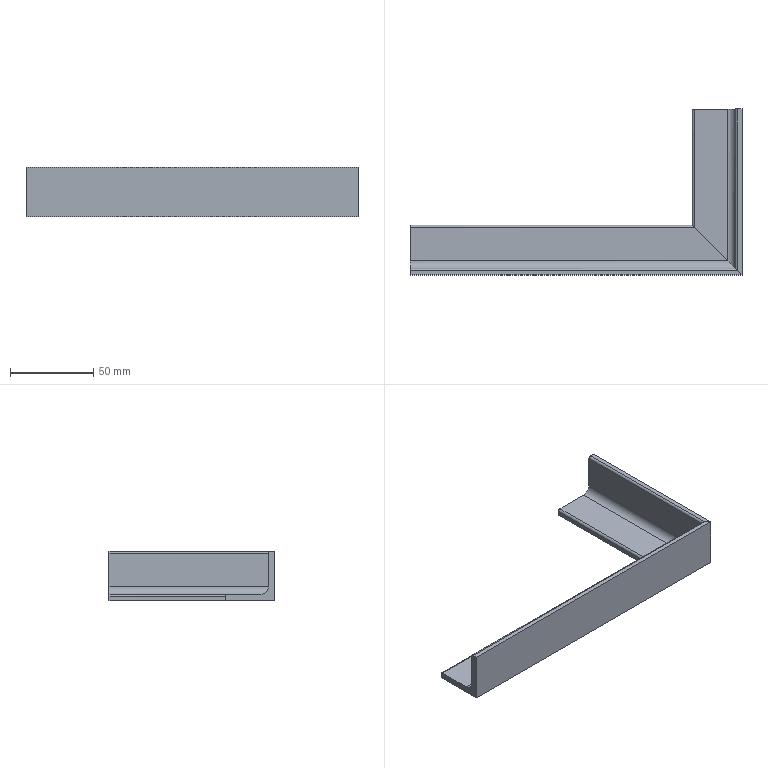Part | SolidWorks | features WeldMemberFeat 1, WeldmentFeature 1 | 2 solids | 22 faces | box 200 x 100 x 30 mm | volume 64241 mm3 | plane 16 | cylinder 6 | commonest cylinder face diameters 2.667 x4 9 x2
STEP:
#1=CARTESIAN_POINT('',(200.,0.,0.));
#2=VERTEX_POINT('',#1);
#3=CARTESIAN_POINT('',(170.,30.,0.));
#4=VERTEX_POINT('',#3);
#5=CARTESIAN_POINT('',(185.,15.,0.));
#6=DIRECTION('',(-0.7071,0.7071,0.));
#7=VECTOR('',#6,1000.);
#8=LINE('',#5,#7);
#9=EDGE_CURVE('',#2,#4,#8,.T.);
#10=ORIENTED_EDGE('',*,*,#9,.F.);
#11=CARTESIAN_POINT('',(0.,0.,0.));
#12=VERTEX_POINT('',#11);
#13=CARTESIAN_POINT('',(200.,0.,0.));
#14=DIRECTION('',(-1.,0.,0.));
#15=VECTOR('',#14,1000.);
#16=LINE('',#13,#15);
#17=EDGE_CURVE('',#2,#12,#16,.T.);
#18=ORIENTED_EDGE('',*,*,#17,.T.);
#19=CARTESIAN_POINT('',(0.,30.,0.));
#20=VERTEX_POINT('',#19);
#21=CARTESIAN_POINT('',(0.,30.,0.));
#22=DIRECTION('',(0.,1.,0.));
#23=VECTOR('',#22,1000.);
#24=LINE('',#21,#23);
#25=EDGE_CURVE('',#12,#20,#24,.T.);
#26=ORIENTED_EDGE('',*,*,#25,.T.);
#27=CARTESIAN_POINT('',(200.,30.,0.));
#28=DIRECTION('',(-1.,0.,0.));
#29=VECTOR('',#28,1000.);
#30=LINE('',#27,#29);
#31=EDGE_CURVE('',#4,#20,#30,.T.);
#32=ORIENTED_EDGE('',*,*,#31,.F.);
#33=EDGE_LOOP('',(#10,#18,#26,#32));
#34=FACE_OUTER_BOUND('',#33,.T.);
#35=CARTESIAN_POINT('',(200.,30.,0.));
#36=DIRECTION('',(0.,0.,1.));
#37=DIRECTION('',(1.,0.,0.));
#38=AXIS2_PLACEMENT_3D('',#35,#36,#37);
#39=PLANE('',#38);
#40=ADVANCED_FACE('',(#34),#39,.F.);
#41=CARTESIAN_POINT('',(170.,30.,2.667));
#42=VERTEX_POINT('',#41);
#43=CARTESIAN_POINT('',(170.,30.,0.));
#44=DIRECTION('',(0.,0.,1.));
#45=VECTOR('',#44,1000.);
#46=LINE('',#43,#45);
#47=EDGE_CURVE('',#4,#42,#46,.T.);
#48=ORIENTED_EDGE('',*,*,#47,.F.);
#49=ORIENTED_EDGE('',*,*,#31,.T.);
#50=CARTESIAN_POINT('',(0.,30.,2.667));
#51=VERTEX_POINT('',#50);
#52=CARTESIAN_POINT('',(0.,30.,0.));
#53=DIRECTION('',(0.,0.,1.));
#54=VECTOR('',#53,1000.);
#55=LINE('',#52,#54);
#56=EDGE_CURVE('',#20,#51,#55,.T.);
#57=ORIENTED_EDGE('',*,*,#56,.T.);
#58=CARTESIAN_POINT('',(200.,30.,2.667));
#59=DIRECTION('',(-1.,0.,0.));
#60=VECTOR('',#59,1000.);
#61=LINE('',#58,#60);
#62=EDGE_CURVE('',#42,#51,#61,.T.);
#63=ORIENTED_EDGE('',*,*,#62,.F.);
#64=EDGE_LOOP('',(#48,#49,#57,#63));
#65=FACE_OUTER_BOUND('',#64,.T.);
#66=CARTESIAN_POINT('',(200.,30.,0.));
#67=DIRECTION('',(0.,-1.,0.));
#68=DIRECTION('',(0.,0.,-1.));
#69=AXIS2_PLACEMENT_3D('',#66,#67,#68);
#70=PLANE('',#69);
#71=ADVANCED_FACE('',(#65),#70,.F.);
#72=CARTESIAN_POINT('',(171.333,28.667,4.));
#73=VERTEX_POINT('',#72);
#74=CARTESIAN_POINT('',(170.,30.,2.667));
#75=CARTESIAN_POINT('',(170.,30.,3.448));
#76=CARTESIAN_POINT('',(170.552,29.448,4.));
#77=CARTESIAN_POINT('',(171.333,28.667,4.));
#78=(BOUNDED_CURVE()B_SPLINE_CURVE(3,(#74,#75,#76,#77),.UNSPECIFIED.,.F.,.T.)B_SPLINE_CURVE_WITH_KNOTS((4,4),(0.,1.571),.UNSPECIFIED.)CURVE()GEOMETRIC_REPRESENTATION_ITEM()RATIONAL_B_SPLINE_CURVE((1.,0.8047,0.8047,1.))REPRESENTATION_ITEM(''));
#79=EDGE_CURVE('',#42,#73,#78,.T.);
#80=ORIENTED_EDGE('',*,*,#79,.F.);
#81=ORIENTED_EDGE('',*,*,#62,.T.);
#82=CARTESIAN_POINT('',(0.,28.667,4.));
#83=VERTEX_POINT('',#82);
#84=CARTESIAN_POINT('',(0.,28.667,2.667));
#85=DIRECTION('',(1.,0.,0.));
#86=DIRECTION('',(0.,0.,-1.));
#87=AXIS2_PLACEMENT_3D('',#84,#85,#86);
#88=CIRCLE('',#87,1.333);
#89=EDGE_CURVE('',#51,#83,#88,.T.);
#90=ORIENTED_EDGE('',*,*,#89,.T.);
#91=CARTESIAN_POINT('',(200.,28.667,4.));
#92=DIRECTION('',(-1.,0.,0.));
#93=VECTOR('',#92,1000.);
#94=LINE('',#91,#93);
#95=EDGE_CURVE('',#73,#83,#94,.T.);
#96=ORIENTED_EDGE('',*,*,#95,.F.);
#97=EDGE_LOOP('',(#80,#81,#90,#96));
#98=FACE_OUTER_BOUND('',#97,.T.);
#99=CARTESIAN_POINT('',(200.,28.667,2.667));
#100=DIRECTION('',(-1.,0.,0.));
#101=DIRECTION('',(0.,0.,1.));
#102=AXIS2_PLACEMENT_3D('',#99,#100,#101);
#103=CYLINDRICAL_SURFACE('',#102,1.333);
#104=ADVANCED_FACE('',(#98),#103,.T.);
#105=CARTESIAN_POINT('',(191.5,8.5,4.));
#106=VERTEX_POINT('',#105);
#107=CARTESIAN_POINT('',(195.75,4.25,4.));
#108=DIRECTION('',(0.7071,-0.7071,0.));
#109=VECTOR('',#108,1000.);
#110=LINE('',#107,#109);
#111=EDGE_CURVE('',#73,#106,#110,.T.);
#112=ORIENTED_EDGE('',*,*,#111,.F.);
#113=ORIENTED_EDGE('',*,*,#95,.T.);
#114=CARTESIAN_POINT('',(0.,8.5,4.));
#115=VERTEX_POINT('',#114);
#116=CARTESIAN_POINT('',(0.,8.5,4.));
#117=DIRECTION('',(0.,-1.,0.));
#118=VECTOR('',#117,1000.);
#119=LINE('',#116,#118);
#120=EDGE_CURVE('',#83,#115,#119,.T.);
#121=ORIENTED_EDGE('',*,*,#120,.T.);
#122=CARTESIAN_POINT('',(200.,8.5,4.));
#123=DIRECTION('',(-1.,0.,0.));
#124=VECTOR('',#123,1000.);
#125=LINE('',#122,#124);
#126=EDGE_CURVE('',#106,#115,#125,.T.);
#127=ORIENTED_EDGE('',*,*,#126,.F.);
#128=EDGE_LOOP('',(#112,#113,#121,#127));
#129=FACE_OUTER_BOUND('',#128,.T.);
#130=CARTESIAN_POINT('',(200.,8.5,4.));
#131=DIRECTION('',(0.,0.,-1.));
#132=DIRECTION('',(0.,1.,0.));
#133=AXIS2_PLACEMENT_3D('',#130,#131,#132);
#134=PLANE('',#133);
#135=ADVANCED_FACE('',(#129),#134,.F.);
#136=CARTESIAN_POINT('',(196.,4.,8.5));
#137=VERTEX_POINT('',#136);
#138=CARTESIAN_POINT('',(191.5,8.5,4.));
#139=CARTESIAN_POINT('',(194.136,5.864,4.));
#140=CARTESIAN_POINT('',(196.,4.,5.864));
#141=CARTESIAN_POINT('',(196.,4.,8.5));
#142=(BOUNDED_CURVE()B_SPLINE_CURVE(3,(#138,#139,#140,#141),.UNSPECIFIED.,.F.,.T.)B_SPLINE_CURVE_WITH_KNOTS((4,4),(1.571,3.142),.UNSPECIFIED.)CURVE()GEOMETRIC_REPRESENTATION_ITEM()RATIONAL_B_SPLINE_CURVE((1.,0.8047,0.8047,1.))REPRESENTATION_ITEM(''));
#143=EDGE_CURVE('',#106,#137,#142,.T.);
#144=ORIENTED_EDGE('',*,*,#143,.F.);
#145=ORIENTED_EDGE('',*,*,#126,.T.);
#146=CARTESIAN_POINT('',(0.,4.,8.5));
#147=VERTEX_POINT('',#146);
#148=CARTESIAN_POINT('',(0.,8.5,8.5));
#149=DIRECTION('',(-1.,0.,0.));
#150=DIRECTION('',(0.,0.,1.));
#151=AXIS2_PLACEMENT_3D('',#148,#149,#150);
#152=CIRCLE('',#151,4.5);
#153=EDGE_CURVE('',#115,#147,#152,.T.);
#154=ORIENTED_EDGE('',*,*,#153,.T.);
#155=CARTESIAN_POINT('',(200.,4.,8.5));
#156=DIRECTION('',(-1.,0.,0.));
#157=VECTOR('',#156,1000.);
#158=LINE('',#155,#157);
#159=EDGE_CURVE('',#137,#147,#158,.T.);
#160=ORIENTED_EDGE('',*,*,#159,.F.);
#161=EDGE_LOOP('',(#144,#145,#154,#160));
#162=FACE_OUTER_BOUND('',#161,.T.);
#163=CARTESIAN_POINT('',(200.,8.5,8.5));
#164=DIRECTION('',(-1.,0.,0.));
#165=DIRECTION('',(0.,0.,1.));
#166=AXIS2_PLACEMENT_3D('',#163,#164,#165);
#167=CYLINDRICAL_SURFACE('',#166,4.5);
#168=ADVANCED_FACE('',(#162),#167,.F.);
#169=CARTESIAN_POINT('',(196.,4.,28.667));
#170=VERTEX_POINT('',#169);
#171=CARTESIAN_POINT('',(196.,4.,28.667));
#172=DIRECTION('',(0.,0.,1.));
#173=VECTOR('',#172,1000.);
#174=LINE('',#171,#173);
#175=EDGE_CURVE('',#137,#170,#174,.T.);
#176=ORIENTED_EDGE('',*,*,#175,.F.);
#177=ORIENTED_EDGE('',*,*,#159,.T.);
#178=CARTESIAN_POINT('',(0.,4.,28.667));
#179=VERTEX_POINT('',#178);
#180=CARTESIAN_POINT('',(0.,4.,28.667));
#181=DIRECTION('',(0.,0.,1.));
#182=VECTOR('',#181,1000.);
#183=LINE('',#180,#182);
#184=EDGE_CURVE('',#147,#179,#183,.T.);
#185=ORIENTED_EDGE('',*,*,#184,.T.);
#186=CARTESIAN_POINT('',(200.,4.,28.667));
#187=DIRECTION('',(-1.,0.,0.));
#188=VECTOR('',#187,1000.);
#189=LINE('',#186,#188);
#190=EDGE_CURVE('',#170,#179,#189,.T.);
#191=ORIENTED_EDGE('',*,*,#190,.F.);
#192=EDGE_LOOP('',(#176,#177,#185,#191));
#193=FACE_OUTER_BOUND('',#192,.T.);
#194=CARTESIAN_POINT('',(200.,4.,28.667));
#195=DIRECTION('',(0.,-1.,0.));
#196=DIRECTION('',(0.,0.,-1.));
#197=AXIS2_PLACEMENT_3D('',#194,#195,#196);
#198=PLANE('',#197);
#199=ADVANCED_FACE('',(#193),#198,.F.);
#200=CARTESIAN_POINT('',(197.333,2.667,30.));
#201=VERTEX_POINT('',#200);
#202=CARTESIAN_POINT('',(196.,4.,28.667));
#203=CARTESIAN_POINT('',(196.,4.,29.448));
#204=CARTESIAN_POINT('',(196.552,3.448,30.));
#205=CARTESIAN_POINT('',(197.333,2.667,30.));
#206=(BOUNDED_CURVE()B_SPLINE_CURVE(3,(#202,#203,#204,#205),.UNSPECIFIED.,.F.,.T.)B_SPLINE_CURVE_WITH_KNOTS((4,4),(0.,1.571),.UNSPECIFIED.)CURVE()GEOMETRIC_REPRESENTATION_ITEM()RATIONAL_B_SPLINE_CURVE((1.,0.8047,0.8047,1.))REPRESENTATION_ITEM(''));
#207=EDGE_CURVE('',#170,#201,#206,.T.);
#208=ORIENTED_EDGE('',*,*,#207,.F.);
#209=ORIENTED_EDGE('',*,*,#190,.T.);
#210=CARTESIAN_POINT('',(0.,2.667,30.));
#211=VERTEX_POINT('',#210);
#212=CARTESIAN_POINT('',(0.,2.667,28.667));
#213=DIRECTION('',(1.,0.,0.));
#214=DIRECTION('',(0.,0.,1.));
#215=AXIS2_PLACEMENT_3D('',#212,#213,#214);
#216=CIRCLE('',#215,1.333);
#217=EDGE_CURVE('',#179,#211,#216,.T.);
#218=ORIENTED_EDGE('',*,*,#217,.T.);
#219=CARTESIAN_POINT('',(200.,2.667,30.));
#220=DIRECTION('',(-1.,0.,0.));
#221=VECTOR('',#220,1000.);
#222=LINE('',#219,#221);
#223=EDGE_CURVE('',#201,#211,#222,.T.);
#224=ORIENTED_EDGE('',*,*,#223,.F.);
#225=EDGE_LOOP('',(#208,#209,#218,#224));
#226=FACE_OUTER_BOUND('',#225,.T.);
#227=CARTESIAN_POINT('',(200.,2.667,28.667));
#228=DIRECTION('',(-1.,0.,0.));
#229=DIRECTION('',(0.,0.,1.));
#230=AXIS2_PLACEMENT_3D('',#227,#228,#229);
#231=CYLINDRICAL_SURFACE('',#230,1.333);
#232=ADVANCED_FACE('',(#226),#231,.T.);
#233=CARTESIAN_POINT('',(200.,0.,30.));
#234=VERTEX_POINT('',#233);
#235=CARTESIAN_POINT('',(200.,0.,30.));
#236=DIRECTION('',(0.7071,-0.7071,0.));
#237=VECTOR('',#236,1000.);
#238=LINE('',#235,#237);
#239=EDGE_CURVE('',#201,#234,#238,.T.);
#240=ORIENTED_EDGE('',*,*,#239,.F.);
#241=ORIENTED_EDGE('',*,*,#223,.T.);
#242=CARTESIAN_POINT('',(0.,0.,30.));
#243=VERTEX_POINT('',#242);
#244=CARTESIAN_POINT('',(0.,0.,30.));
#245=DIRECTION('',(0.,-1.,0.));
#246=VECTOR('',#245,1000.);
#247=LINE('',#244,#246);
#248=EDGE_CURVE('',#211,#243,#247,.T.);
#249=ORIENTED_EDGE('',*,*,#248,.T.);
#250=CARTESIAN_POINT('',(200.,0.,30.));
#251=DIRECTION('',(-1.,0.,0.));
#252=VECTOR('',#251,1000.);
#253=LINE('',#250,#252);
#254=EDGE_CURVE('',#234,#243,#253,.T.);
#255=ORIENTED_EDGE('',*,*,#254,.F.);
#256=EDGE_LOOP('',(#240,#241,#249,#255));
#257=FACE_OUTER_BOUND('',#256,.T.);
#258=CARTESIAN_POINT('',(200.,0.,30.));
#259=DIRECTION('',(0.,0.,-1.));
#260=DIRECTION('',(-1.,0.,0.));
#261=AXIS2_PLACEMENT_3D('',#258,#259,#260);
#262=PLANE('',#261);
#263=ADVANCED_FACE('',(#257),#262,.F.);
#264=CARTESIAN_POINT('',(200.,0.,0.));
#265=DIRECTION('',(0.,0.,-1.));
#266=VECTOR('',#265,1000.);
#267=LINE('',#264,#266);
#268=EDGE_CURVE('',#234,#2,#267,.T.);
#269=ORIENTED_EDGE('',*,*,#268,.F.);
#270=ORIENTED_EDGE('',*,*,#254,.T.);
#271=CARTESIAN_POINT('',(0.,0.,0.));
#272=DIRECTION('',(0.,0.,-1.));
#273=VECTOR('',#272,1000.);
#274=LINE('',#271,#273);
#275=EDGE_CURVE('',#243,#12,#274,.T.);
#276=ORIENTED_EDGE('',*,*,#275,.T.);
#277=ORIENTED_EDGE('',*,*,#17,.F.);
#278=EDGE_LOOP('',(#269,#270,#276,#277));
#279=FACE_OUTER_BOUND('',#278,.T.);
#280=CARTESIAN_POINT('',(200.,0.,0.));
#281=DIRECTION('',(0.,1.,0.));
#282=DIRECTION('',(0.,0.,1.));
#283=AXIS2_PLACEMENT_3D('',#280,#281,#282);
#284=PLANE('',#283);
#285=ADVANCED_FACE('',(#279),#284,.F.);
#286=ORIENTED_EDGE('',*,*,#25,.F.);
#287=ORIENTED_EDGE('',*,*,#275,.F.);
#288=ORIENTED_EDGE('',*,*,#248,.F.);
#289=ORIENTED_EDGE('',*,*,#217,.F.);
#290=ORIENTED_EDGE('',*,*,#184,.F.);
#291=ORIENTED_EDGE('',*,*,#153,.F.);
#292=ORIENTED_EDGE('',*,*,#120,.F.);
#293=ORIENTED_EDGE('',*,*,#89,.F.);
#294=ORIENTED_EDGE('',*,*,#56,.F.);
#295=EDGE_LOOP('',(#286,#287,#288,#289,#290,#291,#292,#293,#294));
#296=FACE_OUTER_BOUND('',#295,.T.);
#297=CARTESIAN_POINT('',(0.,2.667,28.667));
#298=DIRECTION('',(-1.,0.,0.));
#299=DIRECTION('',(0.,0.,1.));
#300=AXIS2_PLACEMENT_3D('',#297,#298,#299);
#301=PLANE('',#300);
#302=ADVANCED_FACE('',(#296),#301,.T.);
#303=ORIENTED_EDGE('',*,*,#268,.T.);
#304=ORIENTED_EDGE('',*,*,#9,.T.);
#305=ORIENTED_EDGE('',*,*,#47,.T.);
#306=ORIENTED_EDGE('',*,*,#79,.T.);
#307=ORIENTED_EDGE('',*,*,#111,.T.);
#308=ORIENTED_EDGE('',*,*,#143,.T.);
#309=ORIENTED_EDGE('',*,*,#175,.T.);
#310=ORIENTED_EDGE('',*,*,#207,.T.);
#311=ORIENTED_EDGE('',*,*,#239,.T.);
#312=EDGE_LOOP('',(#303,#304,#305,#306,#307,#308,#309,#310,#311));
#313=FACE_OUTER_BOUND('',#312,.T.);
#314=CARTESIAN_POINT('',(200.,0.,0.));
#315=DIRECTION('',(0.7071,0.7071,0.));
#316=DIRECTION('',(-0.7071,0.7071,0.));
#317=AXIS2_PLACEMENT_3D('',#314,#315,#316);
#318=PLANE('',#317);
#319=ADVANCED_FACE('',(#313),#318,.T.);
#320=CLOSED_SHELL('',(#40,#71,#104,#135,#168,#199,#232,#263,#285,#302,#319));
#321=MANIFOLD_SOLID_BREP('',#320);
#322=CARTESIAN_POINT('',(170.,30.,0.));
#323=VERTEX_POINT('',#322);
#324=CARTESIAN_POINT('',(200.,0.,0.));
#325=VERTEX_POINT('',#324);
#326=CARTESIAN_POINT('',(135.,65.,0.));
#327=DIRECTION('',(0.7071,-0.7071,0.));
#328=VECTOR('',#327,1000.);
#329=LINE('',#326,#328);
#330=EDGE_CURVE('',#323,#325,#329,.T.);
#331=ORIENTED_EDGE('',*,*,#330,.F.);
#332=CARTESIAN_POINT('',(170.,100.,0.));
#333=VERTEX_POINT('',#332);
#334=CARTESIAN_POINT('',(170.,100.,0.));
#335=DIRECTION('',(0.,-1.,0.));
#336=VECTOR('',#335,1000.);
#337=LINE('',#334,#336);
#338=EDGE_CURVE('',#333,#323,#337,.T.);
#339=ORIENTED_EDGE('',*,*,#338,.F.);
#340=CARTESIAN_POINT('',(200.,100.,0.));
#341=VERTEX_POINT('',#340);
#342=CARTESIAN_POINT('',(170.,100.,0.));
#343=DIRECTION('',(-1.,0.,0.));
#344=VECTOR('',#343,1000.);
#345=LINE('',#342,#344);
#346=EDGE_CURVE('',#341,#333,#345,.T.);
#347=ORIENTED_EDGE('',*,*,#346,.F.);
#348=CARTESIAN_POINT('',(200.,100.,0.));
#349=DIRECTION('',(0.,-1.,0.));
#350=VECTOR('',#349,1000.);
#351=LINE('',#348,#350);
#352=EDGE_CURVE('',#341,#325,#351,.T.);
#353=ORIENTED_EDGE('',*,*,#352,.T.);
#354=EDGE_LOOP('',(#331,#339,#347,#353));
#355=FACE_OUTER_BOUND('',#354,.T.);
#356=CARTESIAN_POINT('',(170.,100.,0.));
#357=DIRECTION('',(0.,0.,1.));
#358=DIRECTION('',(1.,0.,0.));
#359=AXIS2_PLACEMENT_3D('',#356,#357,#358);
#360=PLANE('',#359);
#361=ADVANCED_FACE('',(#355),#360,.F.);
#362=CARTESIAN_POINT('',(170.,30.,2.667));
#363=VERTEX_POINT('',#362);
#364=CARTESIAN_POINT('',(170.,30.,0.));
#365=DIRECTION('',(0.,0.,-1.));
#366=VECTOR('',#365,1000.);
#367=LINE('',#364,#366);
#368=EDGE_CURVE('',#363,#323,#367,.T.);
#369=ORIENTED_EDGE('',*,*,#368,.F.);
#370=CARTESIAN_POINT('',(170.,100.,2.667));
#371=VERTEX_POINT('',#370);
#372=CARTESIAN_POINT('',(170.,100.,2.667));
#373=DIRECTION('',(0.,-1.,0.));
#374=VECTOR('',#373,1000.);
#375=LINE('',#372,#374);
#376=EDGE_CURVE('',#371,#363,#375,.T.);
#377=ORIENTED_EDGE('',*,*,#376,.F.);
#378=CARTESIAN_POINT('',(170.,100.,0.));
#379=DIRECTION('',(0.,0.,1.));
#380=VECTOR('',#379,1000.);
#381=LINE('',#378,#380);
#382=EDGE_CURVE('',#333,#371,#381,.T.);
#383=ORIENTED_EDGE('',*,*,#382,.F.);
#384=ORIENTED_EDGE('',*,*,#338,.T.);
#385=EDGE_LOOP('',(#369,#377,#383,#384));
#386=FACE_OUTER_BOUND('',#385,.T.);
#387=CARTESIAN_POINT('',(170.,100.,0.));
#388=DIRECTION('',(1.,0.,0.));
#389=DIRECTION('',(0.,0.,-1.));
#390=AXIS2_PLACEMENT_3D('',#387,#388,#389);
#391=PLANE('',#390);
#392=ADVANCED_FACE('',(#386),#391,.F.);
#393=CARTESIAN_POINT('',(171.333,28.667,4.));
#394=VERTEX_POINT('',#393);
#395=CARTESIAN_POINT('',(171.333,28.667,4.));
#396=CARTESIAN_POINT('',(170.552,29.448,4.));
#397=CARTESIAN_POINT('',(170.,30.,3.448));
#398=CARTESIAN_POINT('',(170.,30.,2.667));
#399=(BOUNDED_CURVE()B_SPLINE_CURVE(3,(#395,#396,#397,#398),.UNSPECIFIED.,.F.,.T.)B_SPLINE_CURVE_WITH_KNOTS((4,4),(1.571,3.142),.UNSPECIFIED.)CURVE()GEOMETRIC_REPRESENTATION_ITEM()RATIONAL_B_SPLINE_CURVE((1.,0.8047,0.8047,1.))REPRESENTATION_ITEM(''));
#400=EDGE_CURVE('',#394,#363,#399,.T.);
#401=ORIENTED_EDGE('',*,*,#400,.F.);
#402=CARTESIAN_POINT('',(171.333,100.,4.));
#403=VERTEX_POINT('',#402);
#404=CARTESIAN_POINT('',(171.333,100.,4.));
#405=DIRECTION('',(0.,-1.,0.));
#406=VECTOR('',#405,1000.);
#407=LINE('',#404,#406);
#408=EDGE_CURVE('',#403,#394,#407,.T.);
#409=ORIENTED_EDGE('',*,*,#408,.F.);
#410=CARTESIAN_POINT('',(171.333,100.,2.667));
#411=DIRECTION('',(0.,1.,0.));
#412=DIRECTION('',(0.,0.,-1.));
#413=AXIS2_PLACEMENT_3D('',#410,#411,#412);
#414=CIRCLE('',#413,1.333);
#415=EDGE_CURVE('',#371,#403,#414,.T.);
#416=ORIENTED_EDGE('',*,*,#415,.F.);
#417=ORIENTED_EDGE('',*,*,#376,.T.);
#418=EDGE_LOOP('',(#401,#409,#416,#417));
#419=FACE_OUTER_BOUND('',#418,.T.);
#420=CARTESIAN_POINT('',(171.333,100.,2.667));
#421=DIRECTION('',(0.,-1.,0.));
#422=DIRECTION('',(0.,0.,-1.));
#423=AXIS2_PLACEMENT_3D('',#420,#421,#422);
#424=CYLINDRICAL_SURFACE('',#423,1.333);
#425=ADVANCED_FACE('',(#419),#424,.T.);
#426=CARTESIAN_POINT('',(191.5,8.5,4.));
#427=VERTEX_POINT('',#426);
#428=CARTESIAN_POINT('',(145.75,54.25,4.));
#429=DIRECTION('',(-0.7071,0.7071,0.));
#430=VECTOR('',#429,1000.);
#431=LINE('',#428,#430);
#432=EDGE_CURVE('',#427,#394,#431,.T.);
#433=ORIENTED_EDGE('',*,*,#432,.F.);
#434=CARTESIAN_POINT('',(191.5,100.,4.));
#435=VERTEX_POINT('',#434);
#436=CARTESIAN_POINT('',(191.5,100.,4.));
#437=DIRECTION('',(0.,-1.,0.));
#438=VECTOR('',#437,1000.);
#439=LINE('',#436,#438);
#440=EDGE_CURVE('',#435,#427,#439,.T.);
#441=ORIENTED_EDGE('',*,*,#440,.F.);
#442=CARTESIAN_POINT('',(191.5,100.,4.));
#443=DIRECTION('',(1.,0.,0.));
#444=VECTOR('',#443,1000.);
#445=LINE('',#442,#444);
#446=EDGE_CURVE('',#403,#435,#445,.T.);
#447=ORIENTED_EDGE('',*,*,#446,.F.);
#448=ORIENTED_EDGE('',*,*,#408,.T.);
#449=EDGE_LOOP('',(#433,#441,#447,#448));
#450=FACE_OUTER_BOUND('',#449,.T.);
#451=CARTESIAN_POINT('',(191.5,100.,4.));
#452=DIRECTION('',(0.,0.,-1.));
#453=DIRECTION('',(-1.,0.,0.));
#454=AXIS2_PLACEMENT_3D('',#451,#452,#453);
#455=PLANE('',#454);
#456=ADVANCED_FACE('',(#450),#455,.F.);
#457=CARTESIAN_POINT('',(196.,4.,8.5));
#458=VERTEX_POINT('',#457);
#459=CARTESIAN_POINT('',(196.,4.,8.5));
#460=CARTESIAN_POINT('',(196.,4.,5.864));
#461=CARTESIAN_POINT('',(194.136,5.864,4.));
#462=CARTESIAN_POINT('',(191.5,8.5,4.));
#463=(BOUNDED_CURVE()B_SPLINE_CURVE(3,(#459,#460,#461,#462),.UNSPECIFIED.,.F.,.T.)B_SPLINE_CURVE_WITH_KNOTS((4,4),(0.,1.571),.UNSPECIFIED.)CURVE()GEOMETRIC_REPRESENTATION_ITEM()RATIONAL_B_SPLINE_CURVE((1.,0.8047,0.8047,1.))REPRESENTATION_ITEM(''));
#464=EDGE_CURVE('',#458,#427,#463,.T.);
#465=ORIENTED_EDGE('',*,*,#464,.F.);
#466=CARTESIAN_POINT('',(196.,100.,8.5));
#467=VERTEX_POINT('',#466);
#468=CARTESIAN_POINT('',(196.,100.,8.5));
#469=DIRECTION('',(0.,-1.,0.));
#470=VECTOR('',#469,1000.);
#471=LINE('',#468,#470);
#472=EDGE_CURVE('',#467,#458,#471,.T.);
#473=ORIENTED_EDGE('',*,*,#472,.F.);
#474=CARTESIAN_POINT('',(191.5,100.,8.5));
#475=DIRECTION('',(0.,-1.,0.));
#476=DIRECTION('',(0.,0.,1.));
#477=AXIS2_PLACEMENT_3D('',#474,#475,#476);
#478=CIRCLE('',#477,4.5);
#479=EDGE_CURVE('',#435,#467,#478,.T.);
#480=ORIENTED_EDGE('',*,*,#479,.F.);
#481=ORIENTED_EDGE('',*,*,#440,.T.);
#482=EDGE_LOOP('',(#465,#473,#480,#481));
#483=FACE_OUTER_BOUND('',#482,.T.);
#484=CARTESIAN_POINT('',(191.5,100.,8.5));
#485=DIRECTION('',(0.,-1.,0.));
#486=DIRECTION('',(0.,0.,-1.));
#487=AXIS2_PLACEMENT_3D('',#484,#485,#486);
#488=CYLINDRICAL_SURFACE('',#487,4.5);
#489=ADVANCED_FACE('',(#483),#488,.F.);
#490=CARTESIAN_POINT('',(196.,4.,28.667));
#491=VERTEX_POINT('',#490);
#492=CARTESIAN_POINT('',(196.,4.,28.667));
#493=DIRECTION('',(0.,0.,-1.));
#494=VECTOR('',#493,1000.);
#495=LINE('',#492,#494);
#496=EDGE_CURVE('',#491,#458,#495,.T.);
#497=ORIENTED_EDGE('',*,*,#496,.F.);
#498=CARTESIAN_POINT('',(196.,100.,28.667));
#499=VERTEX_POINT('',#498);
#500=CARTESIAN_POINT('',(196.,100.,28.667));
#501=DIRECTION('',(0.,-1.,0.));
#502=VECTOR('',#501,1000.);
#503=LINE('',#500,#502);
#504=EDGE_CURVE('',#499,#491,#503,.T.);
#505=ORIENTED_EDGE('',*,*,#504,.F.);
#506=CARTESIAN_POINT('',(196.,100.,28.667));
#507=DIRECTION('',(0.,0.,1.));
#508=VECTOR('',#507,1000.);
#509=LINE('',#506,#508);
#510=EDGE_CURVE('',#467,#499,#509,.T.);
#511=ORIENTED_EDGE('',*,*,#510,.F.);
#512=ORIENTED_EDGE('',*,*,#472,.T.);
#513=EDGE_LOOP('',(#497,#505,#511,#512));
#514=FACE_OUTER_BOUND('',#513,.T.);
#515=CARTESIAN_POINT('',(196.,100.,28.667));
#516=DIRECTION('',(1.,0.,0.));
#517=DIRECTION('',(0.,0.,-1.));
#518=AXIS2_PLACEMENT_3D('',#515,#516,#517);
#519=PLANE('',#518);
#520=ADVANCED_FACE('',(#514),#519,.F.);
#521=CARTESIAN_POINT('',(197.333,2.667,30.));
#522=VERTEX_POINT('',#521);
#523=CARTESIAN_POINT('',(197.333,2.667,30.));
#524=CARTESIAN_POINT('',(196.552,3.448,30.));
#525=CARTESIAN_POINT('',(196.,4.,29.448));
#526=CARTESIAN_POINT('',(196.,4.,28.667));
#527=(BOUNDED_CURVE()B_SPLINE_CURVE(3,(#523,#524,#525,#526),.UNSPECIFIED.,.F.,.T.)B_SPLINE_CURVE_WITH_KNOTS((4,4),(1.571,3.142),.UNSPECIFIED.)CURVE()GEOMETRIC_REPRESENTATION_ITEM()RATIONAL_B_SPLINE_CURVE((1.,0.8047,0.8047,1.))REPRESENTATION_ITEM(''));
#528=EDGE_CURVE('',#522,#491,#527,.T.);
#529=ORIENTED_EDGE('',*,*,#528,.F.);
#530=CARTESIAN_POINT('',(197.333,100.,30.));
#531=VERTEX_POINT('',#530);
#532=CARTESIAN_POINT('',(197.333,100.,30.));
#533=DIRECTION('',(0.,-1.,0.));
#534=VECTOR('',#533,1000.);
#535=LINE('',#532,#534);
#536=EDGE_CURVE('',#531,#522,#535,.T.);
#537=ORIENTED_EDGE('',*,*,#536,.F.);
#538=CARTESIAN_POINT('',(197.333,100.,28.667));
#539=DIRECTION('',(0.,1.,0.));
#540=DIRECTION('',(0.,0.,1.));
#541=AXIS2_PLACEMENT_3D('',#538,#539,#540);
#542=CIRCLE('',#541,1.333);
#543=EDGE_CURVE('',#499,#531,#542,.T.);
#544=ORIENTED_EDGE('',*,*,#543,.F.);
#545=ORIENTED_EDGE('',*,*,#504,.T.);
#546=EDGE_LOOP('',(#529,#537,#544,#545));
#547=FACE_OUTER_BOUND('',#546,.T.);
#548=CARTESIAN_POINT('',(197.333,100.,28.667));
#549=DIRECTION('',(0.,-1.,0.));
#550=DIRECTION('',(0.,0.,-1.));
#551=AXIS2_PLACEMENT_3D('',#548,#549,#550);
#552=CYLINDRICAL_SURFACE('',#551,1.333);
#553=ADVANCED_FACE('',(#547),#552,.T.);
#554=CARTESIAN_POINT('',(200.,0.,30.));
#555=VERTEX_POINT('',#554);
#556=CARTESIAN_POINT('',(150.,50.,30.));
#557=DIRECTION('',(-0.7071,0.7071,0.));
#558=VECTOR('',#557,1000.);
#559=LINE('',#556,#558);
#560=EDGE_CURVE('',#555,#522,#559,.T.);
#561=ORIENTED_EDGE('',*,*,#560,.F.);
#562=CARTESIAN_POINT('',(200.,100.,30.));
#563=VERTEX_POINT('',#562);
#564=CARTESIAN_POINT('',(200.,100.,30.));
#565=DIRECTION('',(0.,-1.,0.));
#566=VECTOR('',#565,1000.);
#567=LINE('',#564,#566);
#568=EDGE_CURVE('',#563,#555,#567,.T.);
#569=ORIENTED_EDGE('',*,*,#568,.F.);
#570=CARTESIAN_POINT('',(200.,100.,30.));
#571=DIRECTION('',(1.,0.,0.));
#572=VECTOR('',#571,1000.);
#573=LINE('',#570,#572);
#574=EDGE_CURVE('',#531,#563,#573,.T.);
#575=ORIENTED_EDGE('',*,*,#574,.F.);
#576=ORIENTED_EDGE('',*,*,#536,.T.);
#577=EDGE_LOOP('',(#561,#569,#575,#576));
#578=FACE_OUTER_BOUND('',#577,.T.);
#579=CARTESIAN_POINT('',(200.,100.,30.));
#580=DIRECTION('',(0.,0.,-1.));
#581=DIRECTION('',(-1.,0.,0.));
#582=AXIS2_PLACEMENT_3D('',#579,#580,#581);
#583=PLANE('',#582);
#584=ADVANCED_FACE('',(#578),#583,.F.);
#585=CARTESIAN_POINT('',(200.,0.,0.));
#586=DIRECTION('',(0.,0.,1.));
#587=VECTOR('',#586,1000.);
#588=LINE('',#585,#587);
#589=EDGE_CURVE('',#325,#555,#588,.T.);
#590=ORIENTED_EDGE('',*,*,#589,.F.);
#591=ORIENTED_EDGE('',*,*,#352,.F.);
#592=CARTESIAN_POINT('',(200.,100.,0.));
#593=DIRECTION('',(0.,0.,-1.));
#594=VECTOR('',#593,1000.);
#595=LINE('',#592,#594);
#596=EDGE_CURVE('',#563,#341,#595,.T.);
#597=ORIENTED_EDGE('',*,*,#596,.F.);
#598=ORIENTED_EDGE('',*,*,#568,.T.);
#599=EDGE_LOOP('',(#590,#591,#597,#598));
#600=FACE_OUTER_BOUND('',#599,.T.);
#601=CARTESIAN_POINT('',(200.,100.,0.));
#602=DIRECTION('',(-1.,0.,0.));
#603=DIRECTION('',(0.,0.,1.));
#604=AXIS2_PLACEMENT_3D('',#601,#602,#603);
#605=PLANE('',#604);
#606=ADVANCED_FACE('',(#600),#605,.F.);
#607=ORIENTED_EDGE('',*,*,#346,.T.);
#608=ORIENTED_EDGE('',*,*,#382,.T.);
#609=ORIENTED_EDGE('',*,*,#415,.T.);
#610=ORIENTED_EDGE('',*,*,#446,.T.);
#611=ORIENTED_EDGE('',*,*,#479,.T.);
#612=ORIENTED_EDGE('',*,*,#510,.T.);
#613=ORIENTED_EDGE('',*,*,#543,.T.);
#614=ORIENTED_EDGE('',*,*,#574,.T.);
#615=ORIENTED_EDGE('',*,*,#596,.T.);
#616=EDGE_LOOP('',(#607,#608,#609,#610,#611,#612,#613,#614,#615));
#617=FACE_OUTER_BOUND('',#616,.T.);
#618=CARTESIAN_POINT('',(197.333,100.,28.667));
#619=DIRECTION('',(0.,-1.,0.));
#620=DIRECTION('',(0.,0.,1.));
#621=AXIS2_PLACEMENT_3D('',#618,#619,#620);
#622=PLANE('',#621);
#623=ADVANCED_FACE('',(#617),#622,.F.);
#624=ORIENTED_EDGE('',*,*,#368,.T.);
#625=ORIENTED_EDGE('',*,*,#330,.T.);
#626=ORIENTED_EDGE('',*,*,#589,.T.);
#627=ORIENTED_EDGE('',*,*,#560,.T.);
#628=ORIENTED_EDGE('',*,*,#528,.T.);
#629=ORIENTED_EDGE('',*,*,#496,.T.);
#630=ORIENTED_EDGE('',*,*,#464,.T.);
#631=ORIENTED_EDGE('',*,*,#432,.T.);
#632=ORIENTED_EDGE('',*,*,#400,.T.);
#633=EDGE_LOOP('',(#624,#625,#626,#627,#628,#629,#630,#631,#632));
#634=FACE_OUTER_BOUND('',#633,.T.);
#635=CARTESIAN_POINT('',(200.,0.,0.));
#636=DIRECTION('',(-0.7071,-0.7071,0.));
#637=DIRECTION('',(0.7071,-0.7071,0.));
#638=AXIS2_PLACEMENT_3D('',#635,#636,#637);
#639=PLANE('',#638);
#640=ADVANCED_FACE('',(#634),#639,.T.);
#641=CLOSED_SHELL('',(#361,#392,#425,#456,#489,#520,#553,#584,#606,#623,#640));
#642=MANIFOLD_SOLID_BREP('',#641);
#643=CARTESIAN_POINT('',(0.,0.,0.));
#644=DIRECTION('',(0.,0.,1.));
#645=DIRECTION('',(1.,0.,0.));
#646=AXIS2_PLACEMENT_3D('',#643,#644,#645);
#647=(LENGTH_UNIT()NAMED_UNIT(*)SI_UNIT(.MILLI.,.METRE.));
#648=UNCERTAINTY_MEASURE_WITH_UNIT(LENGTH_MEASURE(0.00001),#647,'','');
#649=(NAMED_UNIT(*)PLANE_ANGLE_UNIT()SI_UNIT($,.RADIAN.));
#650=(NAMED_UNIT(*)SI_UNIT($,.STERADIAN.)SOLID_ANGLE_UNIT());
#651=(GEOMETRIC_REPRESENTATION_CONTEXT(3)GLOBAL_UNCERTAINTY_ASSIGNED_CONTEXT((#648))GLOBAL_UNIT_ASSIGNED_CONTEXT((#647,#649,#650))REPRESENTATION_CONTEXT('',''));
#652=ADVANCED_BREP_SHAPE_REPRESENTATION('',(#321,#642,#646),#651);